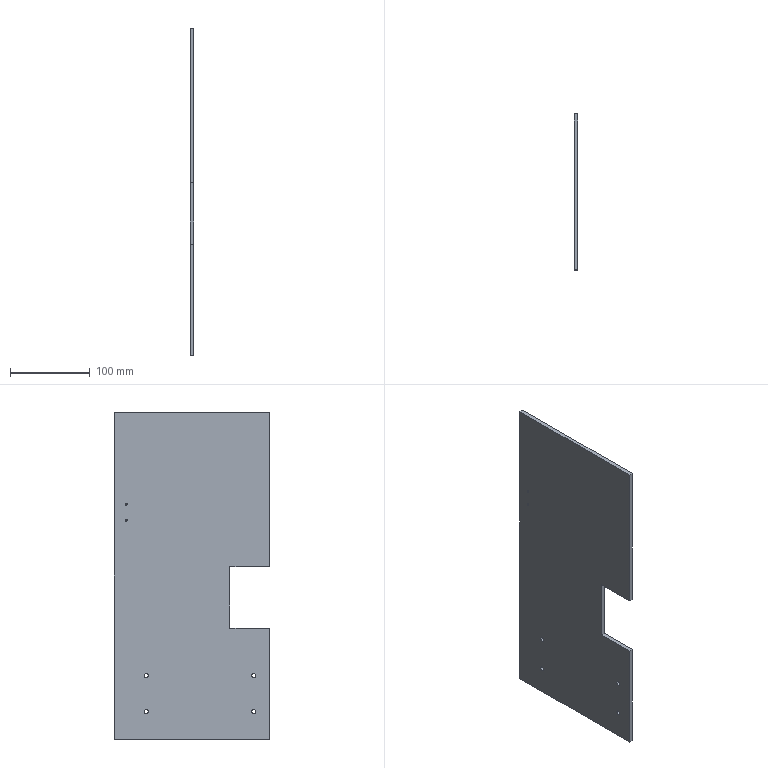Part | STEP file | 09-10 Outer side plate 3 | 1 solid | 22 faces | box 5 x 195 x 410 mm | volume 380058 mm3 | cylinder 12 | plane 10 | commonest cylinder face diameters 5 x8 2.5 x4